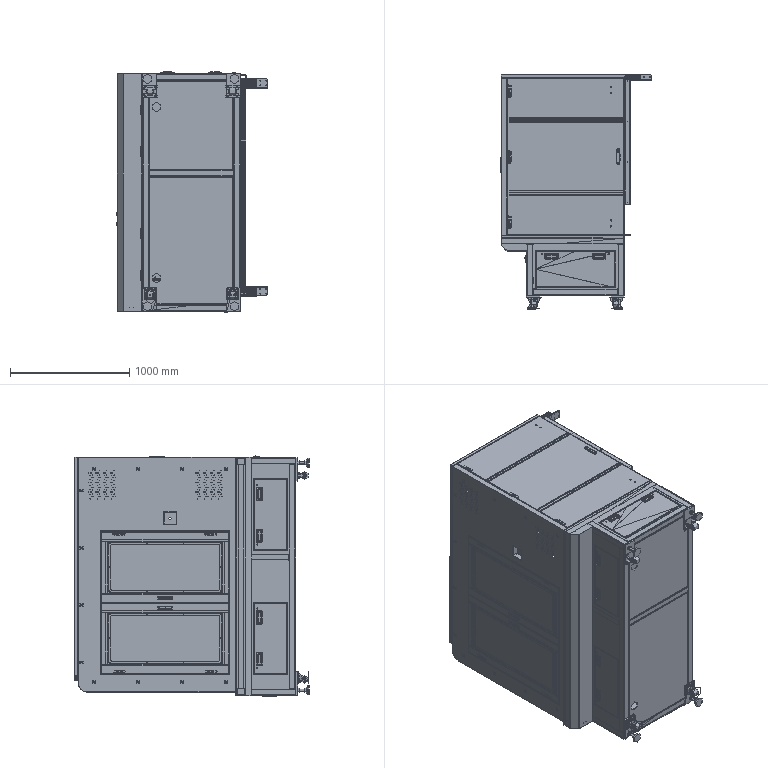Part | NX | features BREP 94 | 160 solids | 11746 faces | volume 13533922777863421821758361749413878049826406618185870581450602983901927865305807591996132092082592415744 mm3 | plane 5861 | cylinder 4933 | cone 420 | torus 284 | spline 248 | commonest cylinder face diameters 1 x764 0.4 x627 4 x472 7 x444 6 x355 5 x272